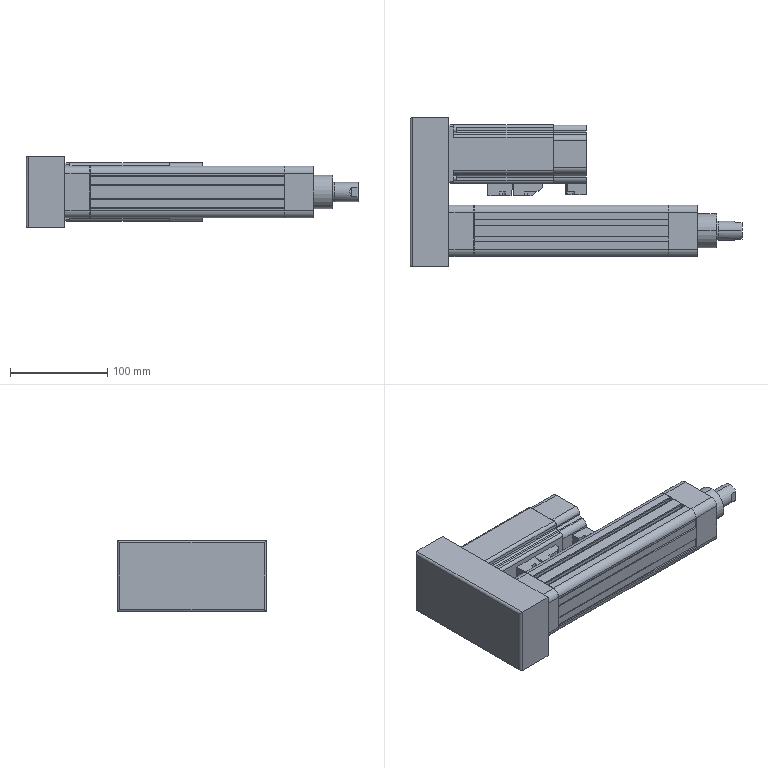Part | SolidWorks | 4 solids | 467 faces | box 342 x 153.7 x 73.7 mm | volume 1636225 mm3 | plane 285 | cylinder 148 | cone 34 | commonest cylinder face diameters 9 x21 6 x20 5.5 x16 2 x12 4 x12 4.917 x8